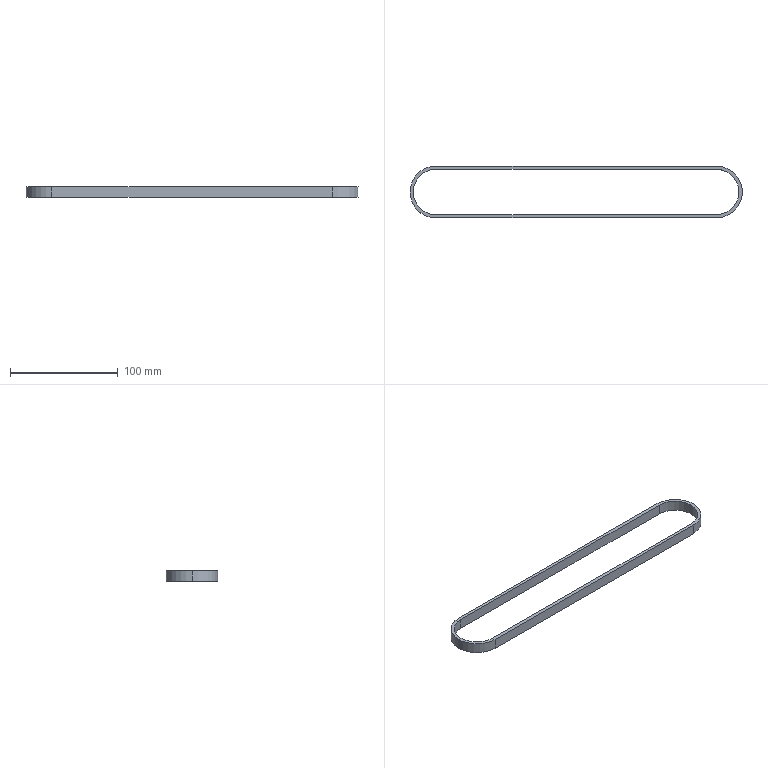Part | SolidWorks | features Extrusion 1, Shell 1 | 1 solid | 12 faces | box 308 x 48 x 10 mm | volume 19841 mm3 | cylinder 6 | plane 6 | commonest cylinder face diameters 42 x3 48 x3
STEP:
#1=CARTESIAN_POINT('',(-260.,21.,10.));
#2=VERTEX_POINT('',#1);
#3=CARTESIAN_POINT('',(-281.,0.,10.));
#4=VERTEX_POINT('',#3);
#5=CARTESIAN_POINT('',(-260.,0.,10.));
#6=DIRECTION('',(0.,0.,1.));
#7=DIRECTION('',(1.,0.,0.));
#8=AXIS2_PLACEMENT_3D('',#5,#6,#7);
#9=CIRCLE('',#8,21.);
#10=EDGE_CURVE('',#2,#4,#9,.T.);
#11=ORIENTED_EDGE('',*,*,#10,.T.);
#12=CARTESIAN_POINT('',(-281.,0.,0.));
#13=VERTEX_POINT('',#12);
#14=CARTESIAN_POINT('',(-281.,0.,10.));
#15=DIRECTION('',(0.,0.,-1.));
#16=VECTOR('',#15,1000.);
#17=LINE('',#14,#16);
#18=EDGE_CURVE('',#4,#13,#17,.T.);
#19=ORIENTED_EDGE('',*,*,#18,.T.);
#20=CARTESIAN_POINT('',(-260.,21.,0.));
#21=VERTEX_POINT('',#20);
#22=CARTESIAN_POINT('',(-260.,0.,0.));
#23=DIRECTION('',(0.,0.,1.));
#24=DIRECTION('',(1.,0.,0.));
#25=AXIS2_PLACEMENT_3D('',#22,#23,#24);
#26=CIRCLE('',#25,21.);
#27=EDGE_CURVE('',#21,#13,#26,.T.);
#28=ORIENTED_EDGE('',*,*,#27,.F.);
#29=CARTESIAN_POINT('',(-260.,21.,10.));
#30=DIRECTION('',(0.,0.,-1.));
#31=VECTOR('',#30,1000.);
#32=LINE('',#29,#31);
#33=EDGE_CURVE('',#2,#21,#32,.T.);
#34=ORIENTED_EDGE('',*,*,#33,.F.);
#35=EDGE_LOOP('',(#11,#19,#28,#34));
#36=FACE_OUTER_BOUND('',#35,.T.);
#37=CARTESIAN_POINT('',(-260.,0.,10.));
#38=DIRECTION('',(0.,0.,-1.));
#39=DIRECTION('',(-1.,0.,0.));
#40=AXIS2_PLACEMENT_3D('',#37,#38,#39);
#41=CYLINDRICAL_SURFACE('',#40,21.);
#42=ADVANCED_FACE('',(#36),#41,.F.);
#43=CARTESIAN_POINT('',(-284.,0.,10.));
#44=VERTEX_POINT('',#43);
#45=CARTESIAN_POINT('',(-260.,-24.,10.));
#46=VERTEX_POINT('',#45);
#47=CARTESIAN_POINT('',(-260.,0.,10.));
#48=DIRECTION('',(0.,0.,1.));
#49=DIRECTION('',(1.,0.,0.));
#50=AXIS2_PLACEMENT_3D('',#47,#48,#49);
#51=CIRCLE('',#50,24.);
#52=EDGE_CURVE('',#44,#46,#51,.T.);
#53=ORIENTED_EDGE('',*,*,#52,.F.);
#54=CARTESIAN_POINT('',(-284.,0.,0.));
#55=VERTEX_POINT('',#54);
#56=CARTESIAN_POINT('',(-284.,0.,10.));
#57=DIRECTION('',(0.,0.,-1.));
#58=VECTOR('',#57,1000.);
#59=LINE('',#56,#58);
#60=EDGE_CURVE('',#44,#55,#59,.T.);
#61=ORIENTED_EDGE('',*,*,#60,.T.);
#62=CARTESIAN_POINT('',(-260.,-24.,0.));
#63=VERTEX_POINT('',#62);
#64=CARTESIAN_POINT('',(-260.,0.,0.));
#65=DIRECTION('',(0.,0.,1.));
#66=DIRECTION('',(1.,0.,0.));
#67=AXIS2_PLACEMENT_3D('',#64,#65,#66);
#68=CIRCLE('',#67,24.);
#69=EDGE_CURVE('',#55,#63,#68,.T.);
#70=ORIENTED_EDGE('',*,*,#69,.T.);
#71=CARTESIAN_POINT('',(-260.,-24.,10.));
#72=DIRECTION('',(0.,0.,-1.));
#73=VECTOR('',#72,1000.);
#74=LINE('',#71,#73);
#75=EDGE_CURVE('',#46,#63,#74,.T.);
#76=ORIENTED_EDGE('',*,*,#75,.F.);
#77=EDGE_LOOP('',(#53,#61,#70,#76));
#78=FACE_OUTER_BOUND('',#77,.T.);
#79=CARTESIAN_POINT('',(-260.,0.,10.));
#80=DIRECTION('',(0.,0.,-1.));
#81=DIRECTION('',(-1.,0.,0.));
#82=AXIS2_PLACEMENT_3D('',#79,#80,#81);
#83=CYLINDRICAL_SURFACE('',#82,24.);
#84=ADVANCED_FACE('',(#78),#83,.T.);
#85=CARTESIAN_POINT('',(0.,-24.,0.));
#86=VERTEX_POINT('',#85);
#87=CARTESIAN_POINT('',(0.,24.,0.));
#88=VERTEX_POINT('',#87);
#89=CARTESIAN_POINT('',(0.,0.,0.));
#90=DIRECTION('',(0.,0.,1.));
#91=DIRECTION('',(1.,0.,0.));
#92=AXIS2_PLACEMENT_3D('',#89,#90,#91);
#93=CIRCLE('',#92,24.);
#94=EDGE_CURVE('',#86,#88,#93,.T.);
#95=ORIENTED_EDGE('',*,*,#94,.T.);
#96=CARTESIAN_POINT('',(0.,24.,10.));
#97=VERTEX_POINT('',#96);
#98=CARTESIAN_POINT('',(0.,24.,10.));
#99=DIRECTION('',(0.,0.,-1.));
#100=VECTOR('',#99,1000.);
#101=LINE('',#98,#100);
#102=EDGE_CURVE('',#97,#88,#101,.T.);
#103=ORIENTED_EDGE('',*,*,#102,.F.);
#104=CARTESIAN_POINT('',(0.,-24.,10.));
#105=VERTEX_POINT('',#104);
#106=CARTESIAN_POINT('',(0.,0.,10.));
#107=DIRECTION('',(0.,0.,1.));
#108=DIRECTION('',(1.,0.,0.));
#109=AXIS2_PLACEMENT_3D('',#106,#107,#108);
#110=CIRCLE('',#109,24.);
#111=EDGE_CURVE('',#105,#97,#110,.T.);
#112=ORIENTED_EDGE('',*,*,#111,.F.);
#113=CARTESIAN_POINT('',(0.,-24.,10.));
#114=DIRECTION('',(0.,0.,-1.));
#115=VECTOR('',#114,1000.);
#116=LINE('',#113,#115);
#117=EDGE_CURVE('',#105,#86,#116,.T.);
#118=ORIENTED_EDGE('',*,*,#117,.T.);
#119=EDGE_LOOP('',(#95,#103,#112,#118));
#120=FACE_OUTER_BOUND('',#119,.T.);
#121=CARTESIAN_POINT('',(0.,0.,10.));
#122=DIRECTION('',(0.,0.,-1.));
#123=DIRECTION('',(-1.,0.,0.));
#124=AXIS2_PLACEMENT_3D('',#121,#122,#123);
#125=CYLINDRICAL_SURFACE('',#124,24.);
#126=ADVANCED_FACE('',(#120),#125,.T.);
#127=CARTESIAN_POINT('',(-260.,24.,0.));
#128=VERTEX_POINT('',#127);
#129=CARTESIAN_POINT('',(0.,24.,0.));
#130=DIRECTION('',(-1.,0.,0.));
#131=VECTOR('',#130,1000.);
#132=LINE('',#129,#131);
#133=EDGE_CURVE('',#88,#128,#132,.T.);
#134=ORIENTED_EDGE('',*,*,#133,.T.);
#135=CARTESIAN_POINT('',(-260.,24.,10.));
#136=VERTEX_POINT('',#135);
#137=CARTESIAN_POINT('',(-260.,24.,10.));
#138=DIRECTION('',(0.,0.,-1.));
#139=VECTOR('',#138,1000.);
#140=LINE('',#137,#139);
#141=EDGE_CURVE('',#136,#128,#140,.T.);
#142=ORIENTED_EDGE('',*,*,#141,.F.);
#143=CARTESIAN_POINT('',(0.,24.,10.));
#144=DIRECTION('',(-1.,0.,0.));
#145=VECTOR('',#144,1000.);
#146=LINE('',#143,#145);
#147=EDGE_CURVE('',#97,#136,#146,.T.);
#148=ORIENTED_EDGE('',*,*,#147,.F.);
#149=ORIENTED_EDGE('',*,*,#102,.T.);
#150=EDGE_LOOP('',(#134,#142,#148,#149));
#151=FACE_OUTER_BOUND('',#150,.T.);
#152=CARTESIAN_POINT('',(0.,24.,10.));
#153=DIRECTION('',(0.,-1.,0.));
#154=DIRECTION('',(0.,0.,-1.));
#155=AXIS2_PLACEMENT_3D('',#152,#153,#154);
#156=PLANE('',#155);
#157=ADVANCED_FACE('',(#151),#156,.F.);
#158=ORIENTED_EDGE('',*,*,#60,.F.);
#159=CARTESIAN_POINT('',(-260.,0.,10.));
#160=DIRECTION('',(0.,0.,1.));
#161=DIRECTION('',(1.,0.,0.));
#162=AXIS2_PLACEMENT_3D('',#159,#160,#161);
#163=CIRCLE('',#162,24.);
#164=EDGE_CURVE('',#136,#44,#163,.T.);
#165=ORIENTED_EDGE('',*,*,#164,.F.);
#166=ORIENTED_EDGE('',*,*,#141,.T.);
#167=CARTESIAN_POINT('',(-260.,0.,0.));
#168=DIRECTION('',(0.,0.,1.));
#169=DIRECTION('',(1.,0.,0.));
#170=AXIS2_PLACEMENT_3D('',#167,#168,#169);
#171=CIRCLE('',#170,24.);
#172=EDGE_CURVE('',#128,#55,#171,.T.);
#173=ORIENTED_EDGE('',*,*,#172,.T.);
#174=EDGE_LOOP('',(#158,#165,#166,#173));
#175=FACE_OUTER_BOUND('',#174,.T.);
#176=CARTESIAN_POINT('',(-260.,0.,10.));
#177=DIRECTION('',(0.,0.,-1.));
#178=DIRECTION('',(-1.,0.,0.));
#179=AXIS2_PLACEMENT_3D('',#176,#177,#178);
#180=CYLINDRICAL_SURFACE('',#179,24.);
#181=ADVANCED_FACE('',(#175),#180,.T.);
#182=CARTESIAN_POINT('',(0.,-24.,0.));
#183=DIRECTION('',(1.,0.,0.));
#184=VECTOR('',#183,1000.);
#185=LINE('',#182,#184);
#186=EDGE_CURVE('',#63,#86,#185,.T.);
#187=ORIENTED_EDGE('',*,*,#186,.T.);
#188=ORIENTED_EDGE('',*,*,#117,.F.);
#189=CARTESIAN_POINT('',(0.,-24.,10.));
#190=DIRECTION('',(1.,0.,0.));
#191=VECTOR('',#190,1000.);
#192=LINE('',#189,#191);
#193=EDGE_CURVE('',#46,#105,#192,.T.);
#194=ORIENTED_EDGE('',*,*,#193,.F.);
#195=ORIENTED_EDGE('',*,*,#75,.T.);
#196=EDGE_LOOP('',(#187,#188,#194,#195));
#197=FACE_OUTER_BOUND('',#196,.T.);
#198=CARTESIAN_POINT('',(0.,-24.,10.));
#199=DIRECTION('',(0.,1.,0.));
#200=DIRECTION('',(0.,0.,1.));
#201=AXIS2_PLACEMENT_3D('',#198,#199,#200);
#202=PLANE('',#201);
#203=ADVANCED_FACE('',(#197),#202,.F.);
#204=CARTESIAN_POINT('',(0.,-21.,10.));
#205=VERTEX_POINT('',#204);
#206=CARTESIAN_POINT('',(0.,21.,10.));
#207=VERTEX_POINT('',#206);
#208=CARTESIAN_POINT('',(0.,0.,10.));
#209=DIRECTION('',(0.,0.,1.));
#210=DIRECTION('',(1.,0.,0.));
#211=AXIS2_PLACEMENT_3D('',#208,#209,#210);
#212=CIRCLE('',#211,21.);
#213=EDGE_CURVE('',#205,#207,#212,.T.);
#214=ORIENTED_EDGE('',*,*,#213,.F.);
#215=CARTESIAN_POINT('',(-260.,-21.,10.));
#216=VERTEX_POINT('',#215);
#217=CARTESIAN_POINT('',(0.,-21.,10.));
#218=DIRECTION('',(1.,0.,0.));
#219=VECTOR('',#218,1000.);
#220=LINE('',#217,#219);
#221=EDGE_CURVE('',#216,#205,#220,.T.);
#222=ORIENTED_EDGE('',*,*,#221,.F.);
#223=CARTESIAN_POINT('',(-260.,0.,10.));
#224=DIRECTION('',(0.,0.,1.));
#225=DIRECTION('',(1.,0.,0.));
#226=AXIS2_PLACEMENT_3D('',#223,#224,#225);
#227=CIRCLE('',#226,21.);
#228=EDGE_CURVE('',#4,#216,#227,.T.);
#229=ORIENTED_EDGE('',*,*,#228,.F.);
#230=ORIENTED_EDGE('',*,*,#10,.F.);
#231=CARTESIAN_POINT('',(0.,21.,10.));
#232=DIRECTION('',(-1.,0.,0.));
#233=VECTOR('',#232,1000.);
#234=LINE('',#231,#233);
#235=EDGE_CURVE('',#207,#2,#234,.T.);
#236=ORIENTED_EDGE('',*,*,#235,.F.);
#237=EDGE_LOOP('',(#214,#222,#229,#230,#236));
#238=FACE_BOUND('',#237,.T.);
#239=ORIENTED_EDGE('',*,*,#111,.T.);
#240=ORIENTED_EDGE('',*,*,#147,.T.);
#241=ORIENTED_EDGE('',*,*,#164,.T.);
#242=ORIENTED_EDGE('',*,*,#52,.T.);
#243=ORIENTED_EDGE('',*,*,#193,.T.);
#244=EDGE_LOOP('',(#239,#240,#241,#242,#243));
#245=FACE_OUTER_BOUND('',#244,.T.);
#246=CARTESIAN_POINT('',(0.,0.,10.));
#247=DIRECTION('',(0.,0.,1.));
#248=DIRECTION('',(1.,0.,0.));
#249=AXIS2_PLACEMENT_3D('',#246,#247,#248);
#250=PLANE('',#249);
#251=ADVANCED_FACE('',(#238,#245),#250,.T.);
#252=CARTESIAN_POINT('',(-260.,-21.,0.));
#253=VERTEX_POINT('',#252);
#254=CARTESIAN_POINT('',(0.,-21.,0.));
#255=VERTEX_POINT('',#254);
#256=CARTESIAN_POINT('',(0.,-21.,0.));
#257=DIRECTION('',(1.,0.,0.));
#258=VECTOR('',#257,1000.);
#259=LINE('',#256,#258);
#260=EDGE_CURVE('',#253,#255,#259,.T.);
#261=ORIENTED_EDGE('',*,*,#260,.T.);
#262=CARTESIAN_POINT('',(0.,21.,0.));
#263=VERTEX_POINT('',#262);
#264=CARTESIAN_POINT('',(0.,0.,0.));
#265=DIRECTION('',(0.,0.,1.));
#266=DIRECTION('',(1.,0.,0.));
#267=AXIS2_PLACEMENT_3D('',#264,#265,#266);
#268=CIRCLE('',#267,21.);
#269=EDGE_CURVE('',#255,#263,#268,.T.);
#270=ORIENTED_EDGE('',*,*,#269,.T.);
#271=CARTESIAN_POINT('',(0.,21.,0.));
#272=DIRECTION('',(-1.,0.,0.));
#273=VECTOR('',#272,1000.);
#274=LINE('',#271,#273);
#275=EDGE_CURVE('',#263,#21,#274,.T.);
#276=ORIENTED_EDGE('',*,*,#275,.T.);
#277=ORIENTED_EDGE('',*,*,#27,.T.);
#278=CARTESIAN_POINT('',(-260.,0.,0.));
#279=DIRECTION('',(0.,0.,1.));
#280=DIRECTION('',(1.,0.,0.));
#281=AXIS2_PLACEMENT_3D('',#278,#279,#280);
#282=CIRCLE('',#281,21.);
#283=EDGE_CURVE('',#13,#253,#282,.T.);
#284=ORIENTED_EDGE('',*,*,#283,.T.);
#285=EDGE_LOOP('',(#261,#270,#276,#277,#284));
#286=FACE_BOUND('',#285,.T.);
#287=ORIENTED_EDGE('',*,*,#94,.F.);
#288=ORIENTED_EDGE('',*,*,#186,.F.);
#289=ORIENTED_EDGE('',*,*,#69,.F.);
#290=ORIENTED_EDGE('',*,*,#172,.F.);
#291=ORIENTED_EDGE('',*,*,#133,.F.);
#292=EDGE_LOOP('',(#287,#288,#289,#290,#291));
#293=FACE_OUTER_BOUND('',#292,.T.);
#294=CARTESIAN_POINT('',(0.,0.,0.));
#295=DIRECTION('',(0.,0.,1.));
#296=DIRECTION('',(1.,0.,0.));
#297=AXIS2_PLACEMENT_3D('',#294,#295,#296);
#298=PLANE('',#297);
#299=ADVANCED_FACE('',(#286,#293),#298,.F.);
#300=ORIENTED_EDGE('',*,*,#269,.F.);
#301=CARTESIAN_POINT('',(0.,-21.,10.));
#302=DIRECTION('',(0.,0.,-1.));
#303=VECTOR('',#302,1000.);
#304=LINE('',#301,#303);
#305=EDGE_CURVE('',#205,#255,#304,.T.);
#306=ORIENTED_EDGE('',*,*,#305,.F.);
#307=ORIENTED_EDGE('',*,*,#213,.T.);
#308=CARTESIAN_POINT('',(0.,21.,10.));
#309=DIRECTION('',(0.,0.,-1.));
#310=VECTOR('',#309,1000.);
#311=LINE('',#308,#310);
#312=EDGE_CURVE('',#207,#263,#311,.T.);
#313=ORIENTED_EDGE('',*,*,#312,.T.);
#314=EDGE_LOOP('',(#300,#306,#307,#313));
#315=FACE_OUTER_BOUND('',#314,.T.);
#316=CARTESIAN_POINT('',(0.,0.,10.));
#317=DIRECTION('',(0.,0.,-1.));
#318=DIRECTION('',(-1.,0.,0.));
#319=AXIS2_PLACEMENT_3D('',#316,#317,#318);
#320=CYLINDRICAL_SURFACE('',#319,21.);
#321=ADVANCED_FACE('',(#315),#320,.F.);
#322=ORIENTED_EDGE('',*,*,#275,.F.);
#323=ORIENTED_EDGE('',*,*,#312,.F.);
#324=ORIENTED_EDGE('',*,*,#235,.T.);
#325=ORIENTED_EDGE('',*,*,#33,.T.);
#326=EDGE_LOOP('',(#322,#323,#324,#325));
#327=FACE_OUTER_BOUND('',#326,.T.);
#328=CARTESIAN_POINT('',(0.,21.,10.));
#329=DIRECTION('',(0.,-1.,0.));
#330=DIRECTION('',(0.,0.,-1.));
#331=AXIS2_PLACEMENT_3D('',#328,#329,#330);
#332=PLANE('',#331);
#333=ADVANCED_FACE('',(#327),#332,.T.);
#334=ORIENTED_EDGE('',*,*,#18,.F.);
#335=ORIENTED_EDGE('',*,*,#228,.T.);
#336=CARTESIAN_POINT('',(-260.,-21.,10.));
#337=DIRECTION('',(0.,0.,-1.));
#338=VECTOR('',#337,1000.);
#339=LINE('',#336,#338);
#340=EDGE_CURVE('',#216,#253,#339,.T.);
#341=ORIENTED_EDGE('',*,*,#340,.T.);
#342=ORIENTED_EDGE('',*,*,#283,.F.);
#343=EDGE_LOOP('',(#334,#335,#341,#342));
#344=FACE_OUTER_BOUND('',#343,.T.);
#345=CARTESIAN_POINT('',(-260.,0.,10.));
#346=DIRECTION('',(0.,0.,-1.));
#347=DIRECTION('',(-1.,0.,0.));
#348=AXIS2_PLACEMENT_3D('',#345,#346,#347);
#349=CYLINDRICAL_SURFACE('',#348,21.);
#350=ADVANCED_FACE('',(#344),#349,.F.);
#351=ORIENTED_EDGE('',*,*,#260,.F.);
#352=ORIENTED_EDGE('',*,*,#340,.F.);
#353=ORIENTED_EDGE('',*,*,#221,.T.);
#354=ORIENTED_EDGE('',*,*,#305,.T.);
#355=EDGE_LOOP('',(#351,#352,#353,#354));
#356=FACE_OUTER_BOUND('',#355,.T.);
#357=CARTESIAN_POINT('',(0.,-21.,10.));
#358=DIRECTION('',(0.,1.,0.));
#359=DIRECTION('',(0.,0.,1.));
#360=AXIS2_PLACEMENT_3D('',#357,#358,#359);
#361=PLANE('',#360);
#362=ADVANCED_FACE('',(#356),#361,.T.);
#363=CLOSED_SHELL('',(#42,#84,#126,#157,#181,#203,#251,#299,#321,#333,#350,#362));
#364=MANIFOLD_SOLID_BREP('',#363);
#365=CARTESIAN_POINT('',(0.,0.,0.));
#366=DIRECTION('',(0.,0.,1.));
#367=DIRECTION('',(1.,0.,0.));
#368=AXIS2_PLACEMENT_3D('',#365,#366,#367);
#369=(LENGTH_UNIT()NAMED_UNIT(*)SI_UNIT(.MILLI.,.METRE.));
#370=UNCERTAINTY_MEASURE_WITH_UNIT(LENGTH_MEASURE(0.00001),#369,'','');
#371=(NAMED_UNIT(*)PLANE_ANGLE_UNIT()SI_UNIT($,.RADIAN.));
#372=(NAMED_UNIT(*)SI_UNIT($,.STERADIAN.)SOLID_ANGLE_UNIT());
#373=(GEOMETRIC_REPRESENTATION_CONTEXT(3)GLOBAL_UNCERTAINTY_ASSIGNED_CONTEXT((#370))GLOBAL_UNIT_ASSIGNED_CONTEXT((#369,#371,#372))REPRESENTATION_CONTEXT('',''));
#374=ADVANCED_BREP_SHAPE_REPRESENTATION('',(#364,#368),#373);